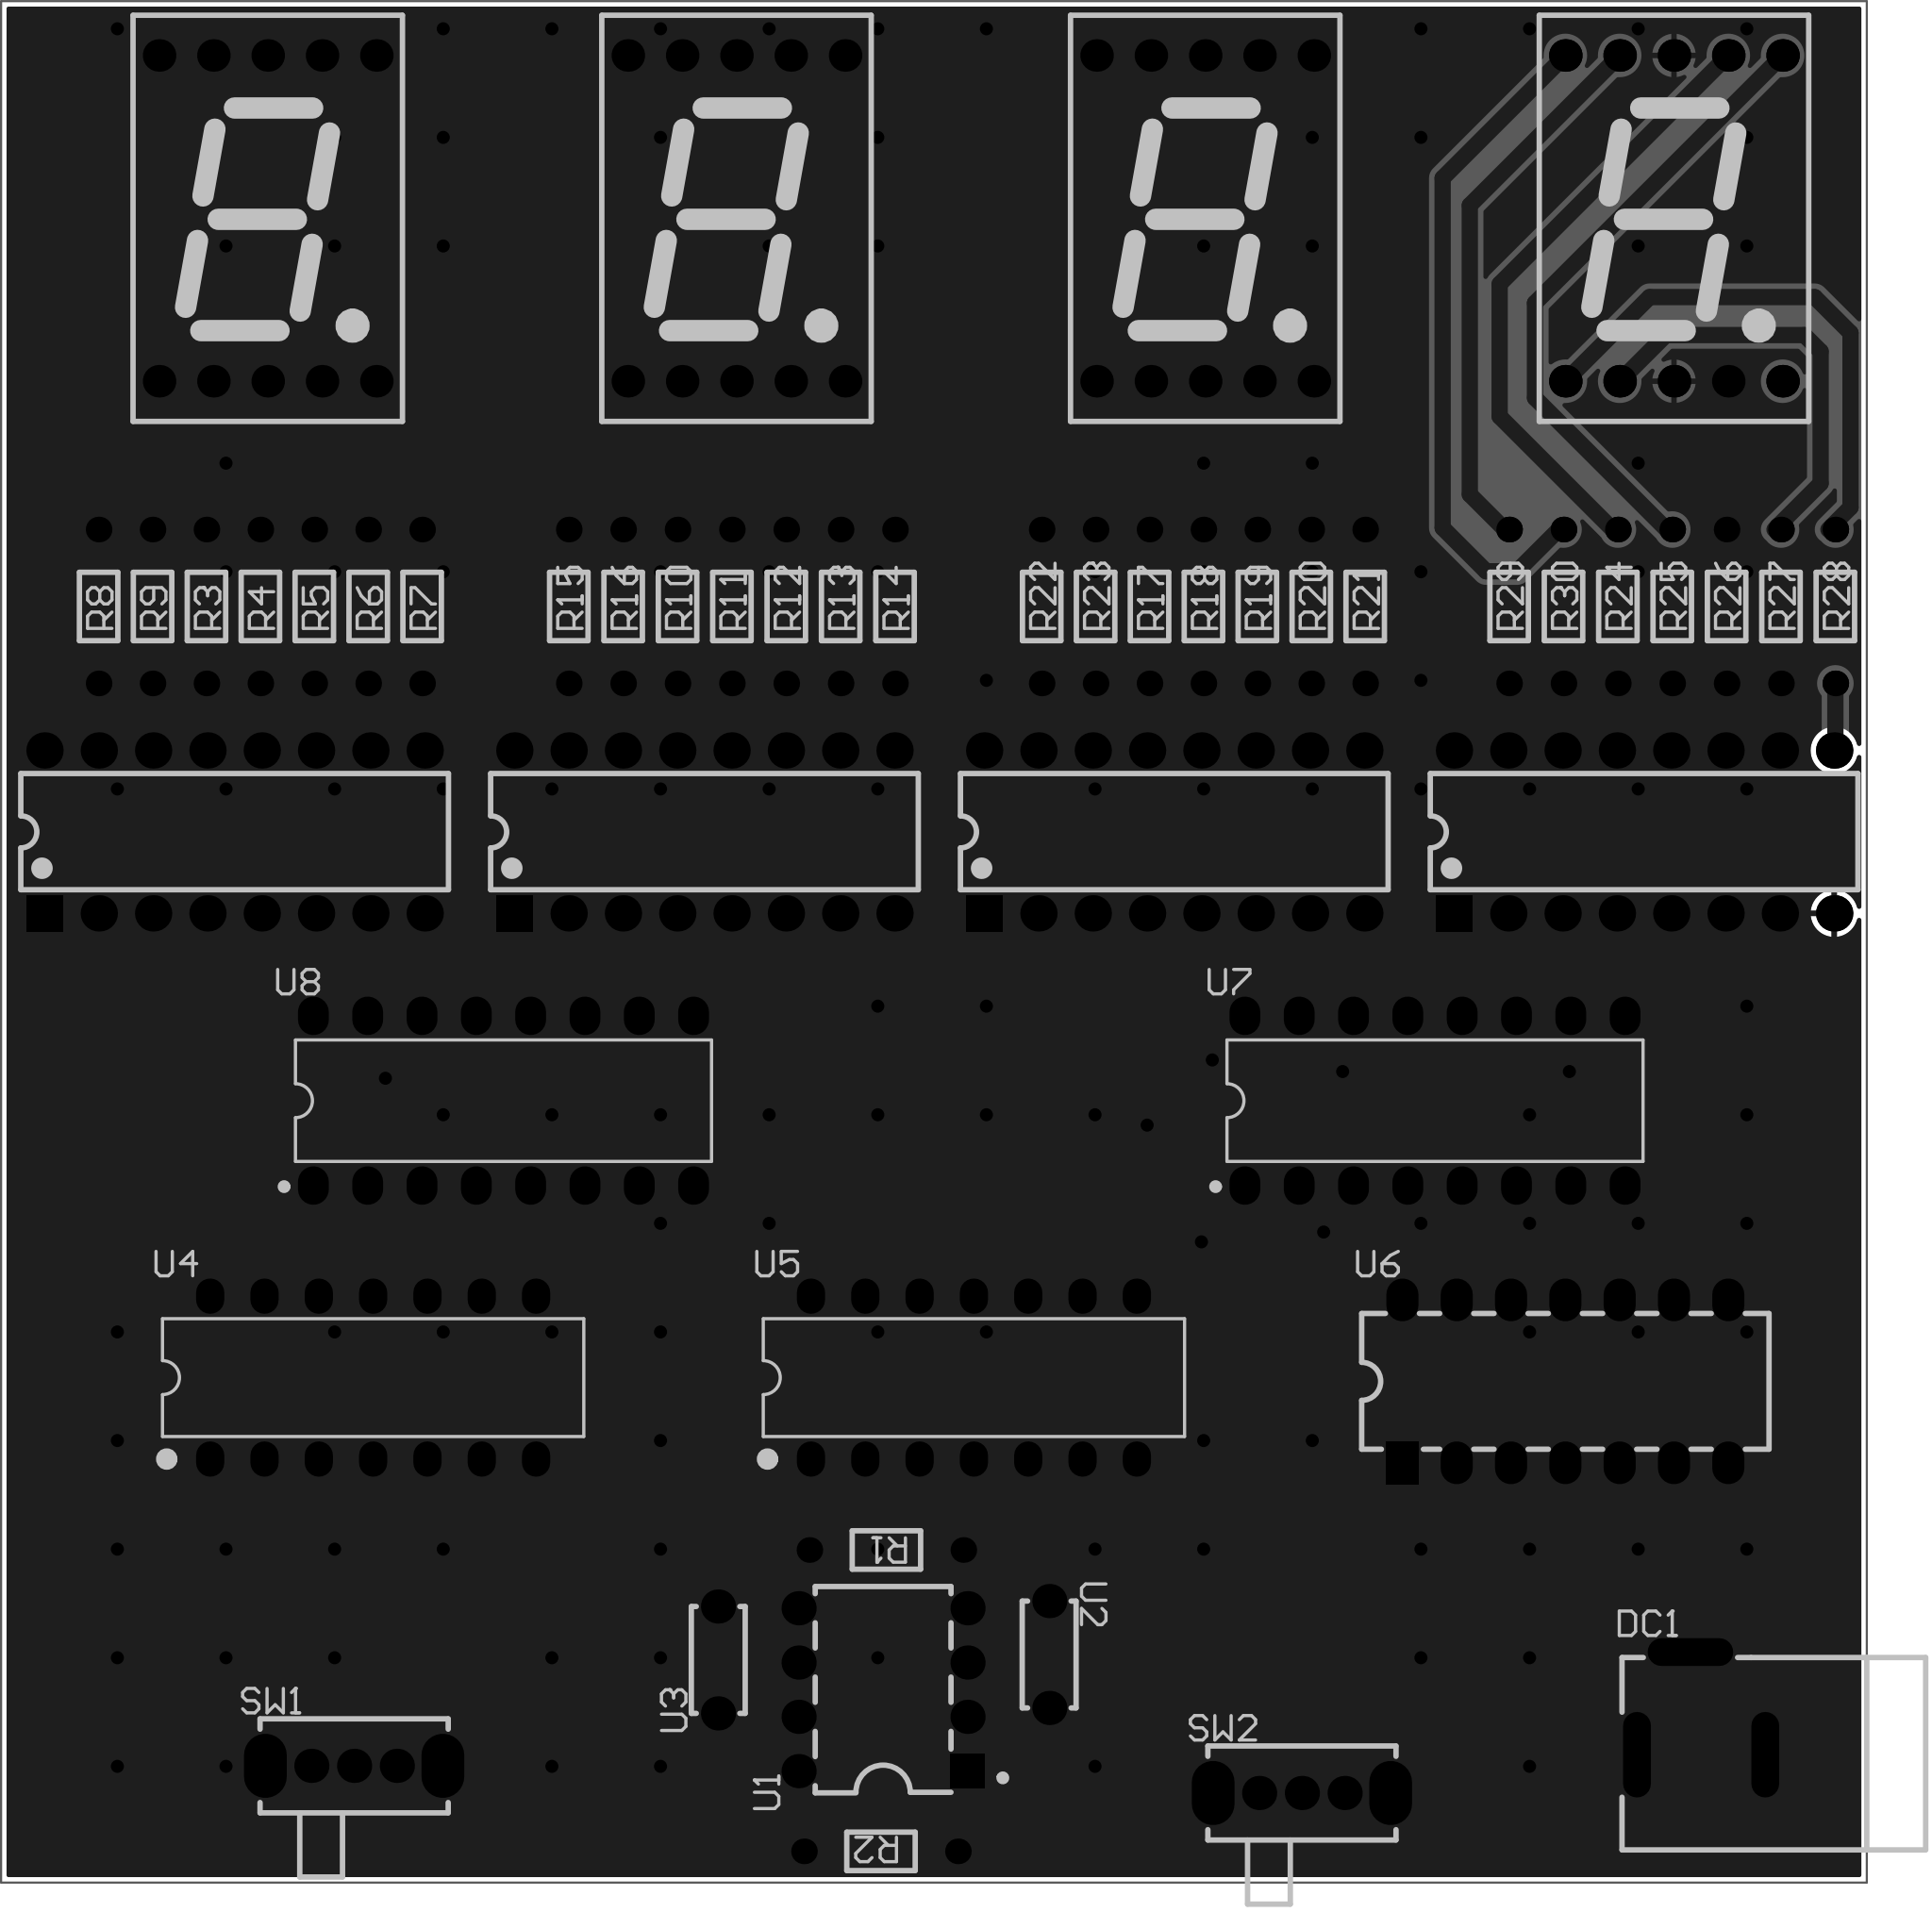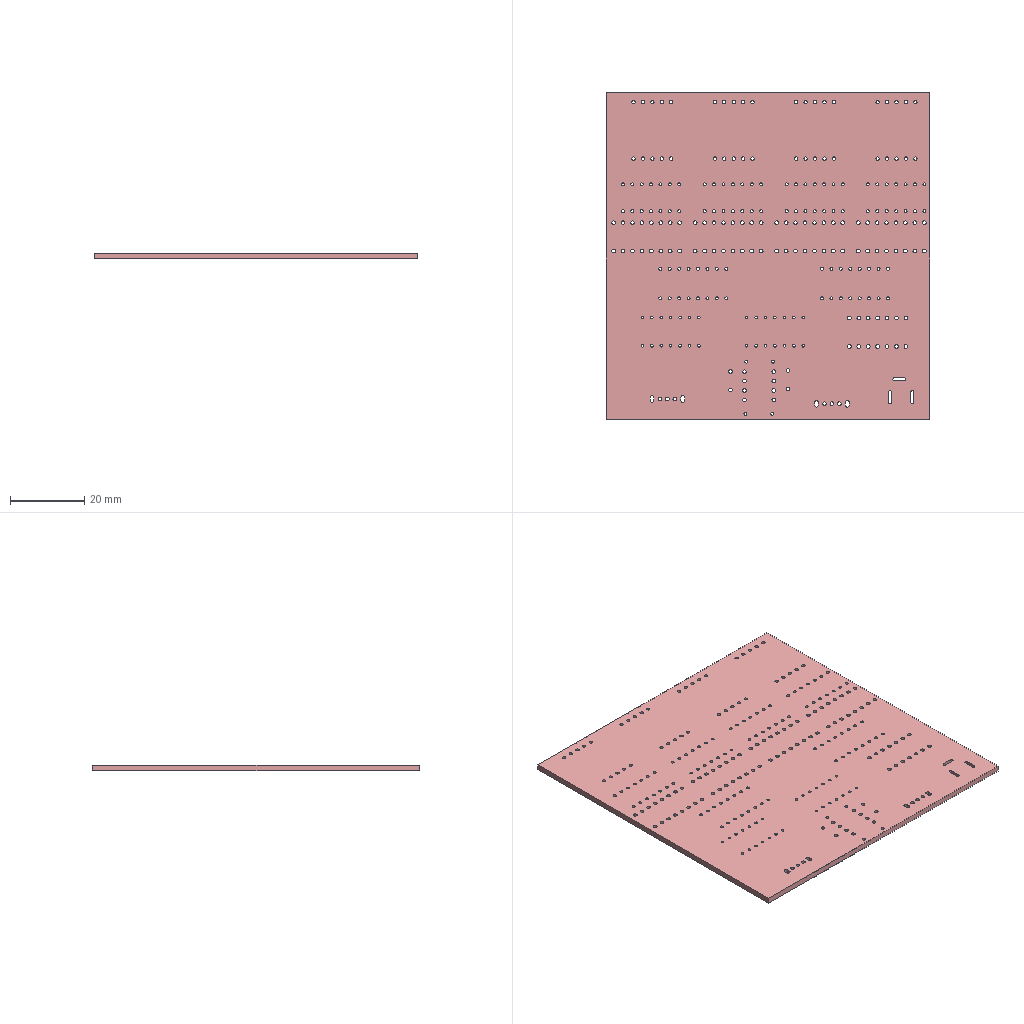Circuit board layout | Altium Designer | box 87.2 x 88 x 1.6 mm
Layer stack:
# Altium Designer layer stack of  (unit mm; dielectric type: 0 none, 1 core, 2 prepreg, 3 surface material)
index,name,kind,layer,copper_thickness_mm,dielectric_type,dielectric_thickness_mm,dielectric_material,dielectric_constant
0,Top Paste Mask Layer,other,,,,,,
1,Top Silkscreen Layer,other,,,,,,
2,Top Solder Mask Layer,dielectric,,,3,0.01,,3.3
3,Top Layer,copper,Top Layer,0.035,,,,
4,Dielectric1,dielectric,,,3,1.51,FR4,4.5
5,Bottom Layer,copper,Bottom Layer,0.035,,,,
6,Bottom Solder Mask Layer,dielectric,,,3,0.01,,3.3
7,Bottom Silkscreen Layer,other,,,,,,
8,Bottom Paste Mask Layer,other,,,,,,
# drill layer pairs: low layer,high layer
drill_pair,Top Layer,Bottom Layer
Part placement:
Designator,Comment,Layer,Footprint,Center-X(mm),Center-Y(mm),Rotation
DC1,,TopLayer,DC-2.0,165.354,98.298,0
LED1,,TopLayer,LED-SEG-TH_10P-L12.6-W19.0-P2.54-S15.24-BL,164.084,167.767,0
LED2,,TopLayer,LED-SEG-TH_10P-L12.6-W19.0-P2.54-S15.24-BL,142.163,167.767,0
LED3,,TopLayer,LED-SEG-TH_10P-L12.6-W19.0-P2.54-S15.24-BL,120.243,167.767,0
LED4,,TopLayer,LED-SEG-TH_10P-L12.6-W19.0-P2.54-S15.24-BL,98.323,167.767,0
R1,68kΩ,TopLayer,Res_1/8W,127.254,105.474,0
R2,10kΩ,TopLayer,Res_1/8W,127,91.377,0
SW1,,TopLayer,拨动开关_侧,102.362,95.377,0
SW2,,TopLayer,拨动开关_侧,146.685,94.107,0
U1,NE555PE4,TopLayer,PDIP-8_L9.6-W6.4-P2.54-LS7.9-BL-1,127.099,98.939,90
U2,100nF,TopLayer,CAP-TH_L5.0-W2.5-P5.00-D1.0,134.874,100.585,270
U3,10nF,TopLayer,CAP-TH_L5.0-W2.5-P5.00-D1.0,119.38,100.331,90
U4,NTE74LS08,TopLayer,DIP-14_L19.6-W6.4-P2.54-LS7.6-BL,103.251,113.538,0
U5,NTE74LS32,TopLayer,DIP-14_L19.6-W6.4-P2.54-LS7.6-BL,131.346,113.538,0
U6,SN74LS00N(XBLW),TopLayer,PDIP-14_L19.3-W6.4-P2.54-LS7.6-BL,159.004,113.363,0
U7,SN74LS390NE4,TopLayer,PDIP-16_L19.3-W6.4-P2.54-LS7.94-BL,152.908,126.492,0
U8,SN74LS390NE4,TopLayer,PDIP-16_L19.3-W6.4-P2.54-LS7.94-BL,109.347,126.492,0
U9,CD74HC4511E,TopLayer,PDIP-16_L19.7-W6.6-P2.54-LS7.6-BL,162.687,139.065,0
U10,CD74HC4511E,TopLayer,PDIP-16_L19.7-W6.6-P2.54-LS7.6-BL,140.716,139.065,0
U11,CD74HC4511E,TopLayer,PDIP-16_L19.7-W6.6-P2.54-LS7.6-BL,118.745,139.065,0
U12,CD74HC4511E,TopLayer,PDIP-16_L19.7-W6.6-P2.54-LS7.6-BL,96.774,139.065,0
R3,300Ω,TopLayer,Res_1/8W,95.457,149.61,90
R4,300Ω,TopLayer,Res_1/8W,97.978,149.61,90
R5,300Ω,TopLayer,Res_1/8W,100.5,149.61,90
R6,300Ω,TopLayer,Res_1/8W,103.021,149.61,90
R7,300Ω,TopLayer,Res_1/8W,105.543,149.61,90
R8,300Ω,TopLayer,Res_1/8W,90.414,149.61,90
R9,300Ω,TopLayer,Res_1/8W,92.935,149.61,90
R10,300Ω,TopLayer,Res_1/8W,117.486,149.61,90
R11,300Ω,TopLayer,Res_1/8W,120.029,149.61,90
R12,300Ω,TopLayer,Res_1/8W,122.571,149.61,90
R13,300Ω,TopLayer,Res_1/8W,125.114,149.61,90
R14,300Ω,TopLayer,Res_1/8W,127.657,149.61,90
R15,300Ω,TopLayer,Res_1/8W,112.401,149.61,90
R16,300Ω,TopLayer,Res_1/8W,114.943,149.61,90
R17,300Ω,TopLayer,Res_1/8W,139.558,149.61,90
R18,300Ω,TopLayer,Res_1/8W,142.079,149.61,90
R19,300Ω,TopLayer,Res_1/8W,144.601,149.61,90
R20,300Ω,TopLayer,Res_1/8W,147.122,149.61,90
R21,300Ω,TopLayer,Res_1/8W,149.644,149.61,90
R22,300Ω,TopLayer,Res_1/8W,134.515,149.61,90
R23,300Ω,TopLayer,Res_1/8W,137.036,149.61,90
R24,300Ω,TopLayer,Res_1/8W,161.46,149.61,90
R25,300Ω,TopLayer,Res_1/8W,164.003,149.61,90
R26,300Ω,TopLayer,Res_1/8W,166.545,149.61,90
R27,300Ω,TopLayer,Res_1/8W,169.088,149.61,90
R28,300Ω,TopLayer,Res_1/8W,171.631,149.61,90
R29,300Ω,TopLayer,Res_1/8W,156.375,149.61,90
R30,300Ω,TopLayer,Res_1/8W,158.917,149.61,90
Pad and via stacks:
# Altium Designer via and pad stacks of  (unit mm). Each distinct definition once, with the count of objects using it.
# via: kind,start_layer,end_layer,hole_mm,diameter_mm,mode(0 simple;1 top-mid-bottom;2 full stack),diameter_per_layer,count,example_net
# pad: kind,layer,hole_mm,hole_type(0 round;1 square;2 slot),plating,top_size,top_shape(1 round;2 rect;3 octagon;9 rounded rect),mid_size,bottom_size,mode,footprint,size_per_layer,count,example
pad,Multi-Layer,0.8001,2,plated,4x1.3,1,4x1.3,4x1.3,0,DC-2.0,,3,DC1.2
pad,Multi-Layer,0.9144,0,plated,1.524x1.524,1,1.524x1.524,1.524x1.524,0,LED-SEG-TH_10P-L12.6-W19.0-P2.54-S15.24-BL,,40,LED1.1
pad,Multi-Layer,0.8001,0,plated,1.199x1.199,1,1.199x1.199,1.199x1.199,0,Res_1/8W,,60,R1.1
pad,Multi-Layer,1.001,0,plated,1.6x1.6,1,1.6x1.6,1.6x1.6,0,\u00B2\u00A6\u00B6\u00AF\u00BF\u00AA\u00B9\u00D8_\u00B2\u00E0,,6,SW1.1
pad,Multi-Layer,1.001,2,plated,3x1.999,1,3x1.999,3x1.999,0,\u00B2\u00A6\u00B6\u00AF\u00BF\u00AA\u00B9\u00D8_\u00B2\u00E0,,4,SW1.4
pad,Multi-Layer,1,0,plated,1.6x1.6,1,1.6x1.6,1.6x1.6,0,PDIP-8_L9.6-W6.4-P2.54-LS7.9-BL-1,,7,U1.8
pad,Multi-Layer,1,0,plated,1.6x1.6,2,1.6x1.6,1.6x1.6,0,PDIP-8_L9.6-W6.4-P2.54-LS7.9-BL-1,,1,U1.1
pad,Multi-Layer,1,0,plated,1.6x1.6,1,1.6x1.6,1.6x1.6,0,CAP-TH_L5.0-W2.5-P5.00-D1.0,,4,U2.1
pad,Multi-Layer,0.7,0,plated,1.32x1.65,1,1.32x1.65,1.32x1.65,0,DIP-14_L19.6-W6.4-P2.54-LS7.6-BL,,28,U4.1
pad,Multi-Layer,1,0,plated,1.5x2,2,1.5x2,1.5x2,0,PDIP-14_L19.3-W6.4-P2.54-LS7.6-BL,,1,U6.1
pad,Multi-Layer,1,0,plated,1.5x2,1,1.5x2,1.5x2,0,PDIP-14_L19.3-W6.4-P2.54-LS7.6-BL,,13,U6.2
pad,Multi-Layer,0.8,0,plated,1.44x1.8,1,1.44x1.8,1.44x1.8,0,PDIP-16_L19.3-W6.4-P2.54-LS7.94-BL,,32,U7.1
pad,Multi-Layer,1,0,plated,1.7x1.7,2,1.7x1.7,1.7x1.7,0,PDIP-16_L19.7-W6.6-P2.54-LS7.6-BL,,4,U9.1
pad,Multi-Layer,1,0,plated,1.7x1.7,1,1.7x1.7,1.7x1.7,0,PDIP-16_L19.7-W6.6-P2.54-LS7.6-BL,,60,U9.2
via,Top Layer,Bottom Layer,0.3048,0.61,0,,125,$1N70
Copper pours:
name,layer,net,type(0 solid;1 hatched;2 none)
Top Layer-GND,Top Layer,GND,0
Bottom Layer-GND,Bottom Layer,GND,0
Design rules, without the lines most boards share:
# Altium Designer design rules of  (exported by Altium Designer, unit mm)
# columns: name | kind | enabled | priority | scope1 | scope2 | descriptor | typed fields (field=value)
creepage | 65 | enabled | 1 | All | All | Creepage Distance Constraint =(0mil) (All),(All) |
copperThickness1oz_2 | 2 | enabled | 2 | All | All | Width Constraint (Min=30mil) (Max=100mil) (Preferred=30mil) (All) |